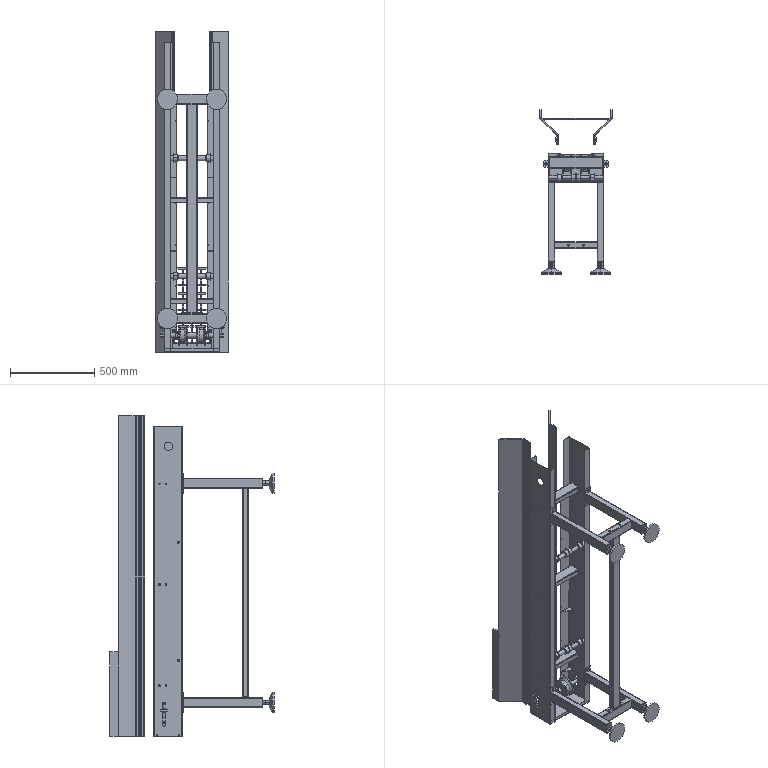Part | SolidWorks | features ReferencePattern 16, LocalLPattern 2, MirrorCompFeat 2 | 114 solids | 2538 faces | box 432 x 974 x 1900 mm | volume 14530091 mm3 | plane 1274 | cone 704 | cylinder 552 | torus 8 | commonest cylinder face diameters 10.5 x100 20 x54 10 x48 8 x46 4.5 x28 4 x24